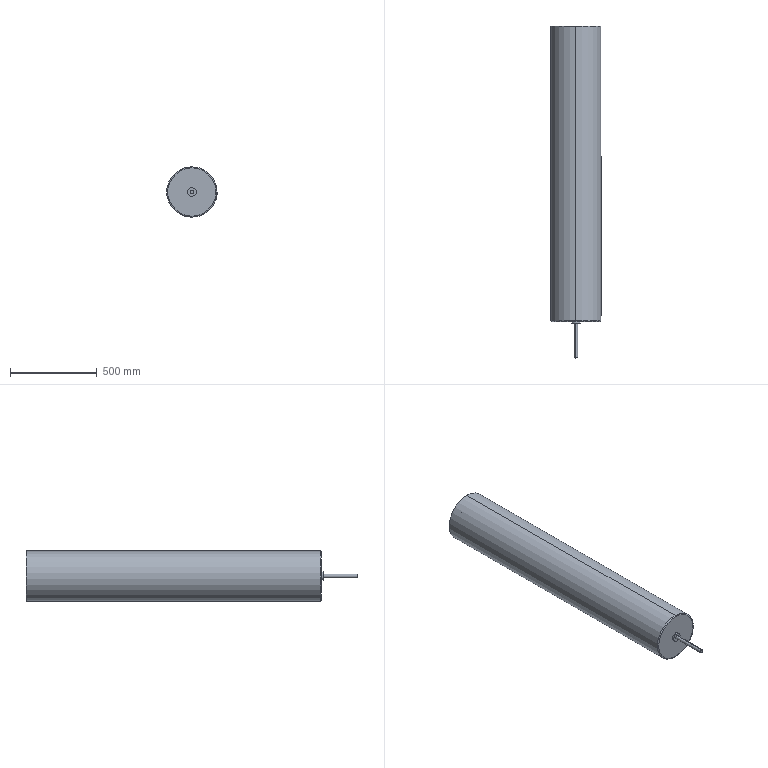Part | SolidWorks | features HoleWzd 3, ICE 2, 3DProfileFeature 1, Revolution 1 | 2 solids | 93 faces | box 290 x 1911 x 290 mm | volume 49235613 mm3 | cylinder 46 | cone 36 | plane 7 | torus 4 | commonest cylinder face diameters 17.5 x32 12 x2 16.5 x2 20 x2 30 x2 50 x2